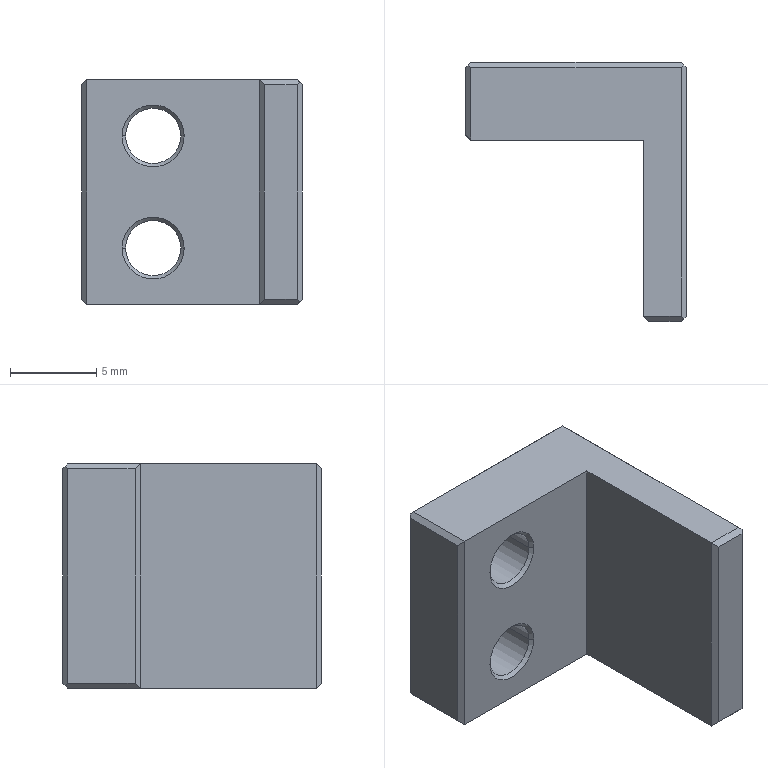Part | NX | 1 solid | 29 faces | box 12.8 x 15 x 13 mm | volume 1011 mm3 | plane 21 | cylinder 4 | cone 4 | commonest cylinder face diameters 3.2 x4
STEP:
#1=CARTESIAN_POINT('',(-175.8,172.2,-82.3));
#2=VERTEX_POINT('',#1);
#3=CARTESIAN_POINT('',(-177.7,172.2,-82.3));
#4=VERTEX_POINT('',#3);
#5=CARTESIAN_POINT('',(-175.,172.2,-82.3));
#6=DIRECTION('',(-1.,0.,0.));
#7=VECTOR('',#6,1000.);
#8=LINE('',#5,#7);
#9=EDGE_CURVE('',#2,#4,#8,.T.);
#10=ORIENTED_EDGE('',*,*,#9,.T.);
#11=CARTESIAN_POINT('',(-177.7,172.2,-94.7));
#12=VERTEX_POINT('',#11);
#13=CARTESIAN_POINT('',(-177.7,172.2,-88.5));
#14=DIRECTION('',(0.,0.,1.));
#15=VECTOR('',#14,1000.);
#16=LINE('',#13,#15);
#17=EDGE_CURVE('',#12,#4,#16,.T.);
#18=ORIENTED_EDGE('',*,*,#17,.F.);
#19=CARTESIAN_POINT('',(-175.8,172.2,-94.7));
#20=VERTEX_POINT('',#19);
#21=CARTESIAN_POINT('',(-175.,172.2,-94.7));
#22=DIRECTION('',(-1.,0.,0.));
#23=VECTOR('',#22,1000.);
#24=LINE('',#21,#23);
#25=EDGE_CURVE('',#20,#12,#24,.T.);
#26=ORIENTED_EDGE('',*,*,#25,.F.);
#27=CARTESIAN_POINT('',(-175.8,172.2,-88.5));
#28=DIRECTION('',(0.,0.,-1.));
#29=VECTOR('',#28,1000.);
#30=LINE('',#27,#29);
#31=EDGE_CURVE('',#2,#20,#30,.T.);
#32=ORIENTED_EDGE('',*,*,#31,.F.);
#33=EDGE_LOOP('',(#10,#18,#26,#32));
#34=FACE_BOUND('',#33,.T.);
#35=CARTESIAN_POINT('',(-175.,172.2,-82.));
#36=DIRECTION('',(0.,-1.,0.));
#37=DIRECTION('',(-1.,0.,0.));
#38=AXIS2_PLACEMENT_3D('',#35,#36,#37);
#39=PLANE('',#38);
#40=ADVANCED_FACE('',(#34),#39,.T.);
#41=CARTESIAN_POINT('',(-175.8,187.2,-94.7));
#42=VERTEX_POINT('',#41);
#43=CARTESIAN_POINT('',(-188.,187.2,-94.7));
#44=VERTEX_POINT('',#43);
#45=CARTESIAN_POINT('',(-175.,187.2,-94.7));
#46=DIRECTION('',(-1.,0.,0.));
#47=VECTOR('',#46,1000.);
#48=LINE('',#45,#47);
#49=EDGE_CURVE('',#42,#44,#48,.T.);
#50=ORIENTED_EDGE('',*,*,#49,.T.);
#51=CARTESIAN_POINT('',(-188.,187.2,-82.3));
#52=VERTEX_POINT('',#51);
#53=CARTESIAN_POINT('',(-188.,187.2,-88.5));
#54=DIRECTION('',(0.,0.,1.));
#55=VECTOR('',#54,1000.);
#56=LINE('',#53,#55);
#57=EDGE_CURVE('',#44,#52,#56,.T.);
#58=ORIENTED_EDGE('',*,*,#57,.T.);
#59=CARTESIAN_POINT('',(-175.8,187.2,-82.3));
#60=VERTEX_POINT('',#59);
#61=CARTESIAN_POINT('',(-175.,187.2,-82.3));
#62=DIRECTION('',(-1.,0.,0.));
#63=VECTOR('',#62,1000.);
#64=LINE('',#61,#63);
#65=EDGE_CURVE('',#60,#52,#64,.T.);
#66=ORIENTED_EDGE('',*,*,#65,.F.);
#67=CARTESIAN_POINT('',(-175.8,187.2,-88.5));
#68=DIRECTION('',(0.,0.,1.));
#69=VECTOR('',#68,1000.);
#70=LINE('',#67,#69);
#71=EDGE_CURVE('',#42,#60,#70,.T.);
#72=ORIENTED_EDGE('',*,*,#71,.F.);
#73=EDGE_LOOP('',(#50,#58,#66,#72));
#74=FACE_BOUND('',#73,.T.);
#75=CARTESIAN_POINT('',(-185.75,187.2,-91.75));
#76=VERTEX_POINT('',#75);
#77=CARTESIAN_POINT('',(-182.55,187.2,-91.75));
#78=VERTEX_POINT('',#77);
#79=CARTESIAN_POINT('',(-184.15,187.2,-91.75));
#80=DIRECTION('',(0.,-1.,0.));
#81=DIRECTION('',(1.,0.,0.));
#82=AXIS2_PLACEMENT_3D('',#79,#80,#81);
#83=CIRCLE('',#82,1.6);
#84=EDGE_CURVE('',#76,#78,#83,.T.);
#85=ORIENTED_EDGE('',*,*,#84,.T.);
#86=CARTESIAN_POINT('',(-184.15,187.2,-91.75));
#87=DIRECTION('',(0.,-1.,0.));
#88=DIRECTION('',(1.,0.,0.));
#89=AXIS2_PLACEMENT_3D('',#86,#87,#88);
#90=CIRCLE('',#89,1.6);
#91=EDGE_CURVE('',#78,#76,#90,.T.);
#92=ORIENTED_EDGE('',*,*,#91,.T.);
#93=EDGE_LOOP('',(#85,#92));
#94=FACE_BOUND('',#93,.T.);
#95=CARTESIAN_POINT('',(-185.75,187.2,-85.25));
#96=VERTEX_POINT('',#95);
#97=CARTESIAN_POINT('',(-182.55,187.2,-85.25));
#98=VERTEX_POINT('',#97);
#99=CARTESIAN_POINT('',(-184.15,187.2,-85.25));
#100=DIRECTION('',(0.,-1.,0.));
#101=DIRECTION('',(1.,0.,0.));
#102=AXIS2_PLACEMENT_3D('',#99,#100,#101);
#103=CIRCLE('',#102,1.6);
#104=EDGE_CURVE('',#96,#98,#103,.T.);
#105=ORIENTED_EDGE('',*,*,#104,.T.);
#106=CARTESIAN_POINT('',(-184.15,187.2,-85.25));
#107=DIRECTION('',(0.,-1.,0.));
#108=DIRECTION('',(1.,0.,0.));
#109=AXIS2_PLACEMENT_3D('',#106,#107,#108);
#110=CIRCLE('',#109,1.6);
#111=EDGE_CURVE('',#98,#96,#110,.T.);
#112=ORIENTED_EDGE('',*,*,#111,.T.);
#113=EDGE_LOOP('',(#105,#112));
#114=FACE_BOUND('',#113,.T.);
#115=CARTESIAN_POINT('',(-190.3,187.2,-95.944));
#116=DIRECTION('',(0.,1.,0.));
#117=DIRECTION('',(0.,0.,-1.));
#118=AXIS2_PLACEMENT_3D('',#115,#116,#117);
#119=PLANE('',#118);
#120=ADVANCED_FACE('',(#74,#94,#114),#119,.T.);
#121=CARTESIAN_POINT('',(-188.3,186.9,-94.7));
#122=VERTEX_POINT('',#121);
#123=CARTESIAN_POINT('',(-188.3,186.9,-82.3));
#124=VERTEX_POINT('',#123);
#125=CARTESIAN_POINT('',(-188.3,186.9,-88.5));
#126=DIRECTION('',(0.,0.,1.));
#127=VECTOR('',#126,1000.);
#128=LINE('',#125,#127);
#129=EDGE_CURVE('',#122,#124,#128,.T.);
#130=ORIENTED_EDGE('',*,*,#129,.F.);
#131=CARTESIAN_POINT('',(-188.3,183.,-94.7));
#132=VERTEX_POINT('',#131);
#133=CARTESIAN_POINT('',(-188.3,184.8,-94.7));
#134=DIRECTION('',(0.,1.,0.));
#135=VECTOR('',#134,1000.);
#136=LINE('',#133,#135);
#137=EDGE_CURVE('',#132,#122,#136,.T.);
#138=ORIENTED_EDGE('',*,*,#137,.F.);
#139=CARTESIAN_POINT('',(-188.3,183.,-82.3));
#140=VERTEX_POINT('',#139);
#141=CARTESIAN_POINT('',(-188.3,183.,-88.5));
#142=DIRECTION('',(0.,0.,-1.));
#143=VECTOR('',#142,1000.);
#144=LINE('',#141,#143);
#145=EDGE_CURVE('',#140,#132,#144,.T.);
#146=ORIENTED_EDGE('',*,*,#145,.F.);
#147=CARTESIAN_POINT('',(-188.3,184.8,-82.3));
#148=DIRECTION('',(0.,1.,0.));
#149=VECTOR('',#148,1000.);
#150=LINE('',#147,#149);
#151=EDGE_CURVE('',#140,#124,#150,.T.);
#152=ORIENTED_EDGE('',*,*,#151,.T.);
#153=EDGE_LOOP('',(#130,#138,#146,#152));
#154=FACE_BOUND('',#153,.T.);
#155=CARTESIAN_POINT('',(-188.3,182.7,-95.944));
#156=DIRECTION('',(-1.,0.,0.));
#157=DIRECTION('',(0.,1.,0.));
#158=AXIS2_PLACEMENT_3D('',#155,#156,#157);
#159=PLANE('',#158);
#160=ADVANCED_FACE('',(#154),#159,.T.);
#161=CARTESIAN_POINT('',(-175.8,172.5,-95.));
#162=VERTEX_POINT('',#161);
#163=CARTESIAN_POINT('',(-178.,172.5,-95.));
#164=VERTEX_POINT('',#163);
#165=CARTESIAN_POINT('',(-175.,172.5,-95.));
#166=DIRECTION('',(-1.,0.,0.));
#167=VECTOR('',#166,1000.);
#168=LINE('',#165,#167);
#169=EDGE_CURVE('',#162,#164,#168,.T.);
#170=ORIENTED_EDGE('',*,*,#169,.T.);
#171=CARTESIAN_POINT('',(-178.,182.7,-95.));
#172=VERTEX_POINT('',#171);
#173=CARTESIAN_POINT('',(-178.,180.866,-95.));
#174=DIRECTION('',(0.,-1.,0.));
#175=VECTOR('',#174,1000.);
#176=LINE('',#173,#175);
#177=EDGE_CURVE('',#172,#164,#176,.T.);
#178=ORIENTED_EDGE('',*,*,#177,.F.);
#179=CARTESIAN_POINT('',(-188.,182.7,-95.));
#180=VERTEX_POINT('',#179);
#181=CARTESIAN_POINT('',(-175.,182.7,-95.));
#182=DIRECTION('',(1.,0.,0.));
#183=VECTOR('',#182,1000.);
#184=LINE('',#181,#183);
#185=EDGE_CURVE('',#180,#172,#184,.T.);
#186=ORIENTED_EDGE('',*,*,#185,.F.);
#187=CARTESIAN_POINT('',(-188.,186.9,-95.));
#188=VERTEX_POINT('',#187);
#189=CARTESIAN_POINT('',(-188.,184.8,-95.));
#190=DIRECTION('',(0.,1.,0.));
#191=VECTOR('',#190,1000.);
#192=LINE('',#189,#191);
#193=EDGE_CURVE('',#180,#188,#192,.T.);
#194=ORIENTED_EDGE('',*,*,#193,.T.);
#195=CARTESIAN_POINT('',(-175.8,186.9,-95.));
#196=VERTEX_POINT('',#195);
#197=CARTESIAN_POINT('',(-175.,186.9,-95.));
#198=DIRECTION('',(-1.,0.,0.));
#199=VECTOR('',#198,1000.);
#200=LINE('',#197,#199);
#201=EDGE_CURVE('',#196,#188,#200,.T.);
#202=ORIENTED_EDGE('',*,*,#201,.F.);
#203=CARTESIAN_POINT('',(-175.8,179.7,-95.));
#204=DIRECTION('',(0.,1.,0.));
#205=VECTOR('',#204,1000.);
#206=LINE('',#203,#205);
#207=EDGE_CURVE('',#162,#196,#206,.T.);
#208=ORIENTED_EDGE('',*,*,#207,.F.);
#209=EDGE_LOOP('',(#170,#178,#186,#194,#202,#208));
#210=FACE_BOUND('',#209,.T.);
#211=CARTESIAN_POINT('',(-176.432,184.505,-95.));
#212=DIRECTION('',(0.,0.,-1.));
#213=DIRECTION('',(-1.,0.,0.));
#214=AXIS2_PLACEMENT_3D('',#211,#212,#213);
#215=PLANE('',#214);
#216=ADVANCED_FACE('',(#210),#215,.T.);
#217=ORIENTED_EDGE('',*,*,#185,.T.);
#218=CARTESIAN_POINT('',(-178.,182.7,-82.));
#219=VERTEX_POINT('',#218);
#220=CARTESIAN_POINT('',(-178.,182.7,-87.033));
#221=DIRECTION('',(0.,0.,1.));
#222=VECTOR('',#221,1000.);
#223=LINE('',#220,#222);
#224=EDGE_CURVE('',#172,#219,#223,.T.);
#225=ORIENTED_EDGE('',*,*,#224,.T.);
#226=CARTESIAN_POINT('',(-188.,182.7,-82.));
#227=VERTEX_POINT('',#226);
#228=CARTESIAN_POINT('',(-175.,182.7,-82.));
#229=DIRECTION('',(1.,0.,0.));
#230=VECTOR('',#229,1000.);
#231=LINE('',#228,#230);
#232=EDGE_CURVE('',#227,#219,#231,.T.);
#233=ORIENTED_EDGE('',*,*,#232,.F.);
#234=CARTESIAN_POINT('',(-188.,182.7,-88.5));
#235=DIRECTION('',(0.,0.,-1.));
#236=VECTOR('',#235,1000.);
#237=LINE('',#234,#236);
#238=EDGE_CURVE('',#227,#180,#237,.T.);
#239=ORIENTED_EDGE('',*,*,#238,.T.);
#240=EDGE_LOOP('',(#217,#225,#233,#239));
#241=FACE_BOUND('',#240,.T.);
#242=CARTESIAN_POINT('',(-185.95,182.7,-85.25));
#243=VERTEX_POINT('',#242);
#244=CARTESIAN_POINT('',(-182.35,182.7,-85.25));
#245=VERTEX_POINT('',#244);
#246=CARTESIAN_POINT('',(-184.15,182.7,-85.25));
#247=DIRECTION('',(0.,-1.,0.));
#248=DIRECTION('',(1.,0.,0.));
#249=AXIS2_PLACEMENT_3D('',#246,#247,#248);
#250=CIRCLE('',#249,1.8);
#251=EDGE_CURVE('',#243,#245,#250,.T.);
#252=ORIENTED_EDGE('',*,*,#251,.F.);
#253=CARTESIAN_POINT('',(-184.15,182.7,-85.25));
#254=DIRECTION('',(0.,-1.,0.));
#255=DIRECTION('',(1.,0.,0.));
#256=AXIS2_PLACEMENT_3D('',#253,#254,#255);
#257=CIRCLE('',#256,1.8);
#258=EDGE_CURVE('',#245,#243,#257,.T.);
#259=ORIENTED_EDGE('',*,*,#258,.F.);
#260=EDGE_LOOP('',(#252,#259));
#261=FACE_BOUND('',#260,.T.);
#262=CARTESIAN_POINT('',(-185.95,182.7,-91.75));
#263=VERTEX_POINT('',#262);
#264=CARTESIAN_POINT('',(-182.35,182.7,-91.75));
#265=VERTEX_POINT('',#264);
#266=CARTESIAN_POINT('',(-184.15,182.7,-91.75));
#267=DIRECTION('',(0.,-1.,0.));
#268=DIRECTION('',(1.,0.,0.));
#269=AXIS2_PLACEMENT_3D('',#266,#267,#268);
#270=CIRCLE('',#269,1.8);
#271=EDGE_CURVE('',#263,#265,#270,.T.);
#272=ORIENTED_EDGE('',*,*,#271,.F.);
#273=CARTESIAN_POINT('',(-184.15,182.7,-91.75));
#274=DIRECTION('',(0.,-1.,0.));
#275=DIRECTION('',(1.,0.,0.));
#276=AXIS2_PLACEMENT_3D('',#273,#274,#275);
#277=CIRCLE('',#276,1.8);
#278=EDGE_CURVE('',#265,#263,#277,.T.);
#279=ORIENTED_EDGE('',*,*,#278,.F.);
#280=EDGE_LOOP('',(#272,#279));
#281=FACE_BOUND('',#280,.T.);
#282=CARTESIAN_POINT('',(-178.,182.7,-95.944));
#283=DIRECTION('',(0.,-1.,0.));
#284=DIRECTION('',(0.,0.,-1.));
#285=AXIS2_PLACEMENT_3D('',#282,#283,#284);
#286=PLANE('',#285);
#287=ADVANCED_FACE('',(#241,#261,#281),#286,.T.);
#288=CARTESIAN_POINT('',(-175.8,172.5,-82.));
#289=VERTEX_POINT('',#288);
#290=CARTESIAN_POINT('',(-175.8,186.9,-82.));
#291=VERTEX_POINT('',#290);
#292=CARTESIAN_POINT('',(-175.8,179.7,-82.));
#293=DIRECTION('',(0.,1.,0.));
#294=VECTOR('',#293,1000.);
#295=LINE('',#292,#294);
#296=EDGE_CURVE('',#289,#291,#295,.T.);
#297=ORIENTED_EDGE('',*,*,#296,.T.);
#298=CARTESIAN_POINT('',(-188.,186.9,-82.));
#299=VERTEX_POINT('',#298);
#300=CARTESIAN_POINT('',(-175.,186.9,-82.));
#301=DIRECTION('',(-1.,0.,0.));
#302=VECTOR('',#301,1000.);
#303=LINE('',#300,#302);
#304=EDGE_CURVE('',#291,#299,#303,.T.);
#305=ORIENTED_EDGE('',*,*,#304,.T.);
#306=CARTESIAN_POINT('',(-188.,184.8,-82.));
#307=DIRECTION('',(0.,1.,0.));
#308=VECTOR('',#307,1000.);
#309=LINE('',#306,#308);
#310=EDGE_CURVE('',#227,#299,#309,.T.);
#311=ORIENTED_EDGE('',*,*,#310,.F.);
#312=ORIENTED_EDGE('',*,*,#232,.T.);
#313=CARTESIAN_POINT('',(-178.,172.5,-82.));
#314=VERTEX_POINT('',#313);
#315=CARTESIAN_POINT('',(-178.,180.866,-82.));
#316=DIRECTION('',(0.,-1.,0.));
#317=VECTOR('',#316,1000.);
#318=LINE('',#315,#317);
#319=EDGE_CURVE('',#219,#314,#318,.T.);
#320=ORIENTED_EDGE('',*,*,#319,.T.);
#321=CARTESIAN_POINT('',(-175.,172.5,-82.));
#322=DIRECTION('',(-1.,0.,0.));
#323=VECTOR('',#322,1000.);
#324=LINE('',#321,#323);
#325=EDGE_CURVE('',#289,#314,#324,.T.);
#326=ORIENTED_EDGE('',*,*,#325,.F.);
#327=EDGE_LOOP('',(#297,#305,#311,#312,#320,#326));
#328=FACE_BOUND('',#327,.T.);
#329=CARTESIAN_POINT('',(-176.432,184.505,-82.));
#330=DIRECTION('',(0.,0.,-1.));
#331=DIRECTION('',(-1.,0.,0.));
#332=AXIS2_PLACEMENT_3D('',#329,#330,#331);
#333=PLANE('',#332);
#334=ADVANCED_FACE('',(#328),#333,.F.);
#335=CARTESIAN_POINT('',(-185.75,182.9,-85.25));
#336=VERTEX_POINT('',#335);
#337=CARTESIAN_POINT('',(-182.55,182.9,-85.25));
#338=VERTEX_POINT('',#337);
#339=CARTESIAN_POINT('',(-184.15,182.9,-85.25));
#340=DIRECTION('',(0.,-1.,0.));
#341=DIRECTION('',(1.,0.,0.));
#342=AXIS2_PLACEMENT_3D('',#339,#340,#341);
#343=CIRCLE('',#342,1.6);
#344=EDGE_CURVE('',#336,#338,#343,.T.);
#345=ORIENTED_EDGE('',*,*,#344,.T.);
#346=CARTESIAN_POINT('',(-182.55,182.7,-85.25));
#347=DIRECTION('',(0.,-1.,0.));
#348=VECTOR('',#347,1000.);
#349=LINE('',#346,#348);
#350=EDGE_CURVE('',#98,#338,#349,.T.);
#351=ORIENTED_EDGE('',*,*,#350,.F.);
#352=ORIENTED_EDGE('',*,*,#104,.F.);
#353=CARTESIAN_POINT('',(-185.75,182.7,-85.25));
#354=DIRECTION('',(0.,-1.,0.));
#355=VECTOR('',#354,1000.);
#356=LINE('',#353,#355);
#357=EDGE_CURVE('',#96,#336,#356,.T.);
#358=ORIENTED_EDGE('',*,*,#357,.T.);
#359=EDGE_LOOP('',(#345,#351,#352,#358));
#360=FACE_BOUND('',#359,.T.);
#361=CARTESIAN_POINT('',(-184.15,182.7,-85.25));
#362=DIRECTION('',(0.,-1.,0.));
#363=DIRECTION('',(1.,0.,0.));
#364=AXIS2_PLACEMENT_3D('',#361,#362,#363);
#365=CYLINDRICAL_SURFACE('',#364,1.6);
#366=ADVANCED_FACE('',(#360),#365,.F.);
#367=ORIENTED_EDGE('',*,*,#344,.F.);
#368=CARTESIAN_POINT('',(-185.75,182.9,-85.25));
#369=DIRECTION('',(-0.7071,-0.7071,0.));
#370=VECTOR('',#369,1000.);
#371=LINE('',#368,#370);
#372=EDGE_CURVE('',#336,#243,#371,.T.);
#373=ORIENTED_EDGE('',*,*,#372,.T.);
#374=ORIENTED_EDGE('',*,*,#251,.T.);
#375=CARTESIAN_POINT('',(-182.55,182.9,-85.25));
#376=DIRECTION('',(0.7071,-0.7071,0.));
#377=VECTOR('',#376,1000.);
#378=LINE('',#375,#377);
#379=EDGE_CURVE('',#338,#245,#378,.T.);
#380=ORIENTED_EDGE('',*,*,#379,.F.);
#381=EDGE_LOOP('',(#367,#373,#374,#380));
#382=FACE_BOUND('',#381,.T.);
#383=CARTESIAN_POINT('',(-184.15,182.9,-85.25));
#384=DIRECTION('',(0.,-1.,0.));
#385=DIRECTION('',(1.,0.,0.));
#386=AXIS2_PLACEMENT_3D('',#383,#384,#385);
#387=CONICAL_SURFACE('',#386,1.6,0.7854);
#388=ADVANCED_FACE('',(#382),#387,.F.);
#389=CARTESIAN_POINT('',(-185.75,182.9,-91.75));
#390=VERTEX_POINT('',#389);
#391=CARTESIAN_POINT('',(-182.55,182.9,-91.75));
#392=VERTEX_POINT('',#391);
#393=CARTESIAN_POINT('',(-184.15,182.9,-91.75));
#394=DIRECTION('',(0.,-1.,0.));
#395=DIRECTION('',(1.,0.,0.));
#396=AXIS2_PLACEMENT_3D('',#393,#394,#395);
#397=CIRCLE('',#396,1.6);
#398=EDGE_CURVE('',#390,#392,#397,.T.);
#399=ORIENTED_EDGE('',*,*,#398,.T.);
#400=CARTESIAN_POINT('',(-182.55,182.7,-91.75));
#401=DIRECTION('',(0.,-1.,0.));
#402=VECTOR('',#401,1000.);
#403=LINE('',#400,#402);
#404=EDGE_CURVE('',#78,#392,#403,.T.);
#405=ORIENTED_EDGE('',*,*,#404,.F.);
#406=ORIENTED_EDGE('',*,*,#84,.F.);
#407=CARTESIAN_POINT('',(-185.75,182.7,-91.75));
#408=DIRECTION('',(0.,-1.,0.));
#409=VECTOR('',#408,1000.);
#410=LINE('',#407,#409);
#411=EDGE_CURVE('',#76,#390,#410,.T.);
#412=ORIENTED_EDGE('',*,*,#411,.T.);
#413=EDGE_LOOP('',(#399,#405,#406,#412));
#414=FACE_BOUND('',#413,.T.);
#415=CARTESIAN_POINT('',(-184.15,182.7,-91.75));
#416=DIRECTION('',(0.,-1.,0.));
#417=DIRECTION('',(1.,0.,0.));
#418=AXIS2_PLACEMENT_3D('',#415,#416,#417);
#419=CYLINDRICAL_SURFACE('',#418,1.6);
#420=ADVANCED_FACE('',(#414),#419,.F.);
#421=ORIENTED_EDGE('',*,*,#398,.F.);
#422=CARTESIAN_POINT('',(-185.75,182.9,-91.75));
#423=DIRECTION('',(-0.7071,-0.7071,0.));
#424=VECTOR('',#423,1000.);
#425=LINE('',#422,#424);
#426=EDGE_CURVE('',#390,#263,#425,.T.);
#427=ORIENTED_EDGE('',*,*,#426,.T.);
#428=ORIENTED_EDGE('',*,*,#271,.T.);
#429=CARTESIAN_POINT('',(-182.55,182.9,-91.75));
#430=DIRECTION('',(0.7071,-0.7071,0.));
#431=VECTOR('',#430,1000.);
#432=LINE('',#429,#431);
#433=EDGE_CURVE('',#392,#265,#432,.T.);
#434=ORIENTED_EDGE('',*,*,#433,.F.);
#435=EDGE_LOOP('',(#421,#427,#428,#434));
#436=FACE_BOUND('',#435,.T.);
#437=CARTESIAN_POINT('',(-184.15,182.9,-91.75));
#438=DIRECTION('',(0.,-1.,0.));
#439=DIRECTION('',(1.,0.,0.));
#440=AXIS2_PLACEMENT_3D('',#437,#438,#439);
#441=CONICAL_SURFACE('',#440,1.6,0.7854);
#442=ADVANCED_FACE('',(#436),#441,.F.);
#443=ORIENTED_EDGE('',*,*,#169,.F.);
#444=CARTESIAN_POINT('',(-175.65,172.35,-94.85));
#445=VERTEX_POINT('',#444);
#446=CARTESIAN_POINT('',(-184.166,180.866,-103.366));
#447=DIRECTION('',(0.5774,-0.5774,0.5774));
#448=VECTOR('',#447,1000.);
#449=LINE('',#446,#448);
#450=EDGE_CURVE('',#162,#445,#449,.T.);
#451=ORIENTED_EDGE('',*,*,#450,.T.);
#452=CARTESIAN_POINT('',(-167.134,180.866,-103.366));
#453=DIRECTION('',(-0.5774,-0.5774,0.5774));
#454=VECTOR('',#453,1000.);
#455=LINE('',#452,#454);
#456=EDGE_CURVE('',#445,#20,#455,.T.);
#457=ORIENTED_EDGE('',*,*,#456,.T.);
#458=ORIENTED_EDGE('',*,*,#25,.T.);
#459=CARTESIAN_POINT('',(-186.366,180.866,-103.366));
#460=DIRECTION('',(-0.5774,0.5774,-0.5774));
#461=VECTOR('',#460,1000.);
#462=LINE('',#459,#461);
#463=EDGE_CURVE('',#12,#164,#462,.T.);
#464=ORIENTED_EDGE('',*,*,#463,.T.);
#465=EDGE_LOOP('',(#443,#451,#457,#458,#464));
#466=FACE_BOUND('',#465,.T.);
#467=CARTESIAN_POINT('',(-176.5,172.35,-94.85));
#468=DIRECTION('',(0.,0.7071,0.7071));
#469=DIRECTION('',(1.,0.,0.));
#470=AXIS2_PLACEMENT_3D('',#467,#468,#469);
#471=PLANE('',#470);
#472=ADVANCED_FACE('',(#466),#471,.F.);
#473=ORIENTED_EDGE('',*,*,#49,.F.);
#474=CARTESIAN_POINT('',(-175.65,187.05,-94.85));
#475=VERTEX_POINT('',#474);
#476=CARTESIAN_POINT('',(-175.,186.4,-95.5));
#477=DIRECTION('',(0.5774,-0.5774,-0.5774));
#478=VECTOR('',#477,1000.);
#479=LINE('',#476,#478);
#480=EDGE_CURVE('',#42,#475,#479,.T.);
#481=ORIENTED_EDGE('',*,*,#480,.T.);
#482=CARTESIAN_POINT('',(-181.834,180.866,-101.034));
#483=DIRECTION('',(-0.5774,-0.5774,-0.5774));
#484=VECTOR('',#483,1000.);
#485=LINE('',#482,#484);
#486=EDGE_CURVE('',#475,#196,#485,.T.);
#487=ORIENTED_EDGE('',*,*,#486,.T.);
#488=ORIENTED_EDGE('',*,*,#201,.T.);
#489=CARTESIAN_POINT('',(-188.15,187.05,-94.85));
#490=VERTEX_POINT('',#489);
#491=CARTESIAN_POINT('',(-175.,173.9,-108.));
#492=DIRECTION('',(-0.5774,0.5774,0.5774));
#493=VECTOR('',#492,1000.);
#494=LINE('',#491,#493);
#495=EDGE_CURVE('',#188,#490,#494,.T.);
#496=ORIENTED_EDGE('',*,*,#495,.T.);
#497=CARTESIAN_POINT('',(-194.334,180.866,-101.034));
#498=DIRECTION('',(-0.5774,-0.5774,-0.5774));
#499=VECTOR('',#498,1000.);
#500=LINE('',#497,#499);
#501=EDGE_CURVE('',#44,#490,#500,.T.);
#502=ORIENTED_EDGE('',*,*,#501,.F.);
#503=EDGE_LOOP('',(#473,#481,#487,#488,#496,#502));
#504=FACE_BOUND('',#503,.T.);
#505=CARTESIAN_POINT('',(-182.65,187.05,-94.85));
#506=DIRECTION('',(0.,-0.7071,0.7071));
#507=DIRECTION('',(-1.,0.,0.));
#508=AXIS2_PLACEMENT_3D('',#505,#506,#507);
#509=PLANE('',#508);
#510=ADVANCED_FACE('',(#504),#509,.F.);
#511=ORIENTED_EDGE('',*,*,#304,.F.);
#512=CARTESIAN_POINT('',(-175.65,187.05,-82.15));
#513=VERTEX_POINT('',#512);
#514=CARTESIAN_POINT('',(-175.,187.7,-82.8));
#515=DIRECTION('',(0.5774,0.5773,-0.5774));
#516=VECTOR('',#515,1000.);
#517=LINE('',#514,#516);
#518=EDGE_CURVE('',#291,#513,#517,.T.);
#519=ORIENTED_EDGE('',*,*,#518,.T.);
#520=CARTESIAN_POINT('',(-180.533,191.933,-87.033));
#521=DIRECTION('',(0.5773,-0.5773,0.5774));
#522=VECTOR('',#521,1000.);
#523=LINE('',#520,#522);
#524=EDGE_CURVE('',#60,#513,#523,.T.);
#525=ORIENTED_EDGE('',*,*,#524,.F.);
#526=ORIENTED_EDGE('',*,*,#65,.T.);
#527=CARTESIAN_POINT('',(-188.15,187.05,-82.15));
#528=VERTEX_POINT('',#527);
#529=CARTESIAN_POINT('',(-183.267,191.933,-87.033));
#530=DIRECTION('',(-0.5773,-0.5773,0.5774));
#531=VECTOR('',#530,1000.);
#532=LINE('',#529,#531);
#533=EDGE_CURVE('',#52,#528,#532,.T.);
#534=ORIENTED_EDGE('',*,*,#533,.T.);
#535=CARTESIAN_POINT('',(-175.,173.9,-69.));
#536=DIRECTION('',(0.5774,-0.5773,0.5774));
#537=VECTOR('',#536,1000.);
#538=LINE('',#535,#537);
#539=EDGE_CURVE('',#528,#299,#538,.T.);
#540=ORIENTED_EDGE('',*,*,#539,.T.);
#541=EDGE_LOOP('',(#511,#519,#525,#526,#534,#540));
#542=FACE_BOUND('',#541,.T.);
#543=CARTESIAN_POINT('',(-182.65,187.05,-82.15));
#544=DIRECTION('',(0.,0.7071,0.7071));
#545=DIRECTION('',(1.,0.,0.));
#546=AXIS2_PLACEMENT_3D('',#543,#544,#545);
#547=PLANE('',#546);
#548=ADVANCED_FACE('',(#542),#547,.T.);
#549=ORIENTED_EDGE('',*,*,#9,.F.);
#550=CARTESIAN_POINT('',(-175.65,172.35,-82.15));
#551=VERTEX_POINT('',#550);
#552=CARTESIAN_POINT('',(-167.134,180.866,-73.634));
#553=DIRECTION('',(-0.5774,-0.5774,-0.5774));
#554=VECTOR('',#553,1000.);
#555=LINE('',#552,#554);
#556=EDGE_CURVE('',#551,#2,#555,.T.);
#557=ORIENTED_EDGE('',*,*,#556,.F.);
#558=CARTESIAN_POINT('',(-184.166,180.866,-73.634));
#559=DIRECTION('',(-0.5774,0.5774,0.5774));
#560=VECTOR('',#559,1000.);
#561=LINE('',#558,#560);
#562=EDGE_CURVE('',#551,#289,#561,.T.);
#563=ORIENTED_EDGE('',*,*,#562,.T.);
#564=ORIENTED_EDGE('',*,*,#325,.T.);
#565=CARTESIAN_POINT('',(-186.366,180.866,-73.634));
#566=DIRECTION('',(-0.5774,0.5774,0.5774));
#567=VECTOR('',#566,1000.);
#568=LINE('',#565,#567);
#569=EDGE_CURVE('',#4,#314,#568,.T.);
#570=ORIENTED_EDGE('',*,*,#569,.F.);
#571=EDGE_LOOP('',(#549,#557,#563,#564,#570));
#572=FACE_BOUND('',#571,.T.);
#573=CARTESIAN_POINT('',(-176.5,172.35,-82.15));
#574=DIRECTION('',(0.,-0.7071,0.7071));
#575=DIRECTION('',(-1.,0.,0.));
#576=AXIS2_PLACEMENT_3D('',#573,#574,#575);
#577=PLANE('',#576);
#578=ADVANCED_FACE('',(#572),#577,.T.);
#579=ORIENTED_EDGE('',*,*,#145,.T.);
#580=CARTESIAN_POINT('',(-175.,169.7,-108.));
#581=DIRECTION('',(-0.5774,0.5774,0.5774));
#582=VECTOR('',#581,1000.);
#583=LINE('',#580,#582);
#584=EDGE_CURVE('',#180,#132,#583,.T.);
#585=ORIENTED_EDGE('',*,*,#584,.F.);
#586=ORIENTED_EDGE('',*,*,#238,.F.);
#587=CARTESIAN_POINT('',(-175.,169.7,-69.));
#588=DIRECTION('',(-0.5774,0.5774,-0.5774));
#589=VECTOR('',#588,1000.);
#590=LINE('',#587,#589);
#591=EDGE_CURVE('',#227,#140,#590,.T.);
#592=ORIENTED_EDGE('',*,*,#591,.T.);
#593=EDGE_LOOP('',(#579,#585,#586,#592));
#594=FACE_BOUND('',#593,.T.);
#595=CARTESIAN_POINT('',(-188.15,182.85,-88.5));
#596=DIRECTION('',(0.7071,0.7071,0.));
#597=DIRECTION('',(0.,0.,-1.));
#598=AXIS2_PLACEMENT_3D('',#595,#596,#597);
#599=PLANE('',#598);
#600=ADVANCED_FACE('',(#594),#599,.F.);
#601=ORIENTED_EDGE('',*,*,#193,.F.);
#602=ORIENTED_EDGE('',*,*,#584,.T.);
#603=ORIENTED_EDGE('',*,*,#137,.T.);
#604=CARTESIAN_POINT('',(-194.334,180.866,-88.666));
#605=DIRECTION('',(0.5774,0.5774,-0.5774));
#606=VECTOR('',#605,1000.);
#607=LINE('',#604,#606);
#608=EDGE_CURVE('',#122,#490,#607,.T.);
#609=ORIENTED_EDGE('',*,*,#608,.T.);
#610=ORIENTED_EDGE('',*,*,#495,.F.);
#611=EDGE_LOOP('',(#601,#602,#603,#609,#610));
#612=FACE_BOUND('',#611,.T.);
#613=CARTESIAN_POINT('',(-188.15,184.8,-94.85));
#614=DIRECTION('',(-0.7071,0.,-0.7071));
#615=DIRECTION('',(-0.7071,0.,0.7071));
#616=AXIS2_PLACEMENT_3D('',#613,#614,#615);
#617=PLANE('',#616);
#618=ADVANCED_FACE('',(#612),#617,.T.);
#619=ORIENTED_EDGE('',*,*,#129,.T.);
#620=CARTESIAN_POINT('',(-194.334,180.866,-88.334));
#621=DIRECTION('',(-0.5774,-0.5774,-0.5774));
#622=VECTOR('',#621,1000.);
#623=LINE('',#620,#622);
#624=EDGE_CURVE('',#528,#124,#623,.T.);
#625=ORIENTED_EDGE('',*,*,#624,.F.);
#626=ORIENTED_EDGE('',*,*,#533,.F.);
#627=ORIENTED_EDGE('',*,*,#57,.F.);
#628=ORIENTED_EDGE('',*,*,#501,.T.);
#629=ORIENTED_EDGE('',*,*,#608,.F.);
#630=EDGE_LOOP('',(#619,#625,#626,#627,#628,#629));
#631=FACE_BOUND('',#630,.T.);
#632=CARTESIAN_POINT('',(-188.15,187.05,-88.5));
#633=DIRECTION('',(0.7071,-0.7071,0.));
#634=DIRECTION('',(0.,0.,-1.));
#635=AXIS2_PLACEMENT_3D('',#632,#633,#634);
#636=PLANE('',#635);
#637=ADVANCED_FACE('',(#631),#636,.F.);
#638=ORIENTED_EDGE('',*,*,#310,.T.);
#639=ORIENTED_EDGE('',*,*,#539,.F.);
#640=ORIENTED_EDGE('',*,*,#624,.T.);
#641=ORIENTED_EDGE('',*,*,#151,.F.);
#642=ORIENTED_EDGE('',*,*,#591,.F.);
#643=EDGE_LOOP('',(#638,#639,#640,#641,#642));
#644=FACE_BOUND('',#643,.T.);
#645=CARTESIAN_POINT('',(-188.15,184.8,-82.15));
#646=DIRECTION('',(0.7071,0.,-0.7071));
#647=DIRECTION('',(0.,-1.,0.));
#648=AXIS2_PLACEMENT_3D('',#645,#646,#647);
#649=PLANE('',#648);
#650=ADVANCED_FACE('',(#644),#649,.F.);
#651=ORIENTED_EDGE('',*,*,#404,.T.);
#652=CARTESIAN_POINT('',(-184.15,182.9,-91.75));
#653=DIRECTION('',(0.,-1.,0.));
#654=DIRECTION('',(1.,0.,0.));
#655=AXIS2_PLACEMENT_3D('',#652,#653,#654);
#656=CIRCLE('',#655,1.6);
#657=EDGE_CURVE('',#392,#390,#656,.T.);
#658=ORIENTED_EDGE('',*,*,#657,.T.);
#659=ORIENTED_EDGE('',*,*,#411,.F.);
#660=ORIENTED_EDGE('',*,*,#91,.F.);
#661=EDGE_LOOP('',(#651,#658,#659,#660));
#662=FACE_BOUND('',#661,.T.);
#663=CARTESIAN_POINT('',(-184.15,182.7,-91.75));
#664=DIRECTION('',(0.,-1.,0.));
#665=DIRECTION('',(1.,0.,0.));
#666=AXIS2_PLACEMENT_3D('',#663,#664,#665);
#667=CYLINDRICAL_SURFACE('',#666,1.6);
#668=ADVANCED_FACE('',(#662),#667,.F.);
#669=ORIENTED_EDGE('',*,*,#433,.T.);
#670=ORIENTED_EDGE('',*,*,#278,.T.);
#671=ORIENTED_EDGE('',*,*,#426,.F.);
#672=ORIENTED_EDGE('',*,*,#657,.F.);
#673=EDGE_LOOP('',(#669,#670,#671,#672));
#674=FACE_BOUND('',#673,.T.);
#675=CARTESIAN_POINT('',(-184.15,182.9,-91.75));
#676=DIRECTION('',(0.,-1.,0.));
#677=DIRECTION('',(1.,0.,0.));
#678=AXIS2_PLACEMENT_3D('',#675,#676,#677);
#679=CONICAL_SURFACE('',#678,1.6,0.7854);
#680=ADVANCED_FACE('',(#674),#679,.F.);
#681=ORIENTED_EDGE('',*,*,#350,.T.);
#682=CARTESIAN_POINT('',(-184.15,182.9,-85.25));
#683=DIRECTION('',(0.,-1.,0.));
#684=DIRECTION('',(1.,0.,0.));
#685=AXIS2_PLACEMENT_3D('',#682,#683,#684);
#686=CIRCLE('',#685,1.6);
#687=EDGE_CURVE('',#338,#336,#686,.T.);
#688=ORIENTED_EDGE('',*,*,#687,.T.);
#689=ORIENTED_EDGE('',*,*,#357,.F.);
#690=ORIENTED_EDGE('',*,*,#111,.F.);
#691=EDGE_LOOP('',(#681,#688,#689,#690));
#692=FACE_BOUND('',#691,.T.);
#693=CARTESIAN_POINT('',(-184.15,182.7,-85.25));
#694=DIRECTION('',(0.,-1.,0.));
#695=DIRECTION('',(1.,0.,0.));
#696=AXIS2_PLACEMENT_3D('',#693,#694,#695);
#697=CYLINDRICAL_SURFACE('',#696,1.6);
#698=ADVANCED_FACE('',(#692),#697,.F.);
#699=ORIENTED_EDGE('',*,*,#379,.T.);
#700=ORIENTED_EDGE('',*,*,#258,.T.);
#701=ORIENTED_EDGE('',*,*,#372,.F.);
#702=ORIENTED_EDGE('',*,*,#687,.F.);
#703=EDGE_LOOP('',(#699,#700,#701,#702));
#704=FACE_BOUND('',#703,.T.);
#705=CARTESIAN_POINT('',(-184.15,182.9,-85.25));
#706=DIRECTION('',(0.,-1.,0.));
#707=DIRECTION('',(1.,0.,0.));
#708=AXIS2_PLACEMENT_3D('',#705,#706,#707);
#709=CONICAL_SURFACE('',#708,1.6,0.7854);
#710=ADVANCED_FACE('',(#704),#709,.F.);
#711=CARTESIAN_POINT('',(-178.,172.5,-88.5));
#712=DIRECTION('',(0.,0.,1.));
#713=VECTOR('',#712,1000.);
#714=LINE('',#711,#713);
#715=EDGE_CURVE('',#164,#314,#714,.T.);
#716=ORIENTED_EDGE('',*,*,#715,.T.);
#717=ORIENTED_EDGE('',*,*,#319,.F.);
#718=ORIENTED_EDGE('',*,*,#224,.F.);
#719=ORIENTED_EDGE('',*,*,#177,.T.);
#720=EDGE_LOOP('',(#716,#717,#718,#719));
#721=FACE_BOUND('',#720,.T.);
#722=CARTESIAN_POINT('',(-178.,180.866,-87.033));
#723=DIRECTION('',(-1.,0.,0.));
#724=DIRECTION('',(0.,0.,1.));
#725=AXIS2_PLACEMENT_3D('',#722,#723,#724);
#726=PLANE('',#725);
#727=ADVANCED_FACE('',(#721),#726,.T.);
#728=ORIENTED_EDGE('',*,*,#715,.F.);
#729=ORIENTED_EDGE('',*,*,#463,.F.);
#730=ORIENTED_EDGE('',*,*,#17,.T.);
#731=ORIENTED_EDGE('',*,*,#569,.T.);
#732=EDGE_LOOP('',(#728,#729,#730,#731));
#733=FACE_BOUND('',#732,.T.);
#734=CARTESIAN_POINT('',(-177.85,172.35,-88.5));
#735=DIRECTION('',(-0.7071,-0.7071,0.));
#736=DIRECTION('',(-0.7071,0.7071,0.));
#737=AXIS2_PLACEMENT_3D('',#734,#735,#736);
#738=PLANE('',#737);
#739=ADVANCED_FACE('',(#733),#738,.T.);
#740=CARTESIAN_POINT('',(-175.5,172.5,-82.3));
#741=VERTEX_POINT('',#740);
#742=CARTESIAN_POINT('',(-175.5,172.5,-94.7));
#743=VERTEX_POINT('',#742);
#744=CARTESIAN_POINT('',(-175.5,172.5,-88.5));
#745=DIRECTION('',(0.,0.,-1.));
#746=VECTOR('',#745,1000.);
#747=LINE('',#744,#746);
#748=EDGE_CURVE('',#741,#743,#747,.T.);
#749=ORIENTED_EDGE('',*,*,#748,.T.);
#750=CARTESIAN_POINT('',(-175.5,186.9,-94.7));
#751=VERTEX_POINT('',#750);
#752=CARTESIAN_POINT('',(-175.5,179.7,-94.7));
#753=DIRECTION('',(0.,1.,0.));
#754=VECTOR('',#753,1000.);
#755=LINE('',#752,#754);
#756=EDGE_CURVE('',#743,#751,#755,.T.);
#757=ORIENTED_EDGE('',*,*,#756,.T.);
#758=CARTESIAN_POINT('',(-175.5,186.9,-82.3));
#759=VERTEX_POINT('',#758);
#760=CARTESIAN_POINT('',(-175.5,186.9,-88.5));
#761=DIRECTION('',(0.,0.,1.));
#762=VECTOR('',#761,1000.);
#763=LINE('',#760,#762);
#764=EDGE_CURVE('',#751,#759,#763,.T.);
#765=ORIENTED_EDGE('',*,*,#764,.T.);
#766=CARTESIAN_POINT('',(-175.5,179.7,-82.3));
#767=DIRECTION('',(0.,1.,0.));
#768=VECTOR('',#767,1000.);
#769=LINE('',#766,#768);
#770=EDGE_CURVE('',#741,#759,#769,.T.);
#771=ORIENTED_EDGE('',*,*,#770,.F.);
#772=EDGE_LOOP('',(#749,#757,#765,#771));
#773=FACE_BOUND('',#772,.T.);
#774=CARTESIAN_POINT('',(-175.5,180.866,-87.033));
#775=DIRECTION('',(-1.,0.,0.));
#776=DIRECTION('',(0.,0.,1.));
#777=AXIS2_PLACEMENT_3D('',#774,#775,#776);
#778=PLANE('',#777);
#779=ADVANCED_FACE('',(#773),#778,.F.);
#780=ORIENTED_EDGE('',*,*,#770,.T.);
#781=CARTESIAN_POINT('',(-175.,186.4,-82.8));
#782=DIRECTION('',(-0.5774,0.5774,0.5774));
#783=VECTOR('',#782,1000.);
#784=LINE('',#781,#783);
#785=EDGE_CURVE('',#759,#513,#784,.T.);
#786=ORIENTED_EDGE('',*,*,#785,.T.);
#787=ORIENTED_EDGE('',*,*,#518,.F.);
#788=ORIENTED_EDGE('',*,*,#296,.F.);
#789=ORIENTED_EDGE('',*,*,#562,.F.);
#790=CARTESIAN_POINT('',(-167.134,180.866,-90.666));
#791=DIRECTION('',(0.5774,0.5774,-0.5774));
#792=VECTOR('',#791,1000.);
#793=LINE('',#790,#792);
#794=EDGE_CURVE('',#551,#741,#793,.T.);
#795=ORIENTED_EDGE('',*,*,#794,.T.);
#796=EDGE_LOOP('',(#780,#786,#787,#788,#789,#795));
#797=FACE_BOUND('',#796,.T.);
#798=CARTESIAN_POINT('',(-175.65,179.7,-82.15));
#799=DIRECTION('',(-0.7071,0.,-0.7071));
#800=DIRECTION('',(-0.7071,0.,0.7071));
#801=AXIS2_PLACEMENT_3D('',#798,#799,#800);
#802=PLANE('',#801);
#803=ADVANCED_FACE('',(#797),#802,.F.);
#804=ORIENTED_EDGE('',*,*,#764,.F.);
#805=CARTESIAN_POINT('',(-175.,186.4,-94.2));
#806=DIRECTION('',(0.5774,-0.5774,0.5774));
#807=VECTOR('',#806,1000.);
#808=LINE('',#805,#807);
#809=EDGE_CURVE('',#475,#751,#808,.T.);
#810=ORIENTED_EDGE('',*,*,#809,.F.);
#811=ORIENTED_EDGE('',*,*,#480,.F.);
#812=ORIENTED_EDGE('',*,*,#71,.T.);
#813=ORIENTED_EDGE('',*,*,#524,.T.);
#814=ORIENTED_EDGE('',*,*,#785,.F.);
#815=EDGE_LOOP('',(#804,#810,#811,#812,#813,#814));
#816=FACE_BOUND('',#815,.T.);
#817=CARTESIAN_POINT('',(-175.65,187.05,-88.5));
#818=DIRECTION('',(0.7071,0.7071,0.));
#819=DIRECTION('',(0.,0.,-1.));
#820=AXIS2_PLACEMENT_3D('',#817,#818,#819);
#821=PLANE('',#820);
#822=ADVANCED_FACE('',(#816),#821,.T.);
#823=ORIENTED_EDGE('',*,*,#756,.F.);
#824=CARTESIAN_POINT('',(-167.134,180.866,-86.334));
#825=DIRECTION('',(0.5774,0.5774,0.5774));
#826=VECTOR('',#825,1000.);
#827=LINE('',#824,#826);
#828=EDGE_CURVE('',#445,#743,#827,.T.);
#829=ORIENTED_EDGE('',*,*,#828,.F.);
#830=ORIENTED_EDGE('',*,*,#450,.F.);
#831=ORIENTED_EDGE('',*,*,#207,.T.);
#832=ORIENTED_EDGE('',*,*,#486,.F.);
#833=ORIENTED_EDGE('',*,*,#809,.T.);
#834=EDGE_LOOP('',(#823,#829,#830,#831,#832,#833));
#835=FACE_BOUND('',#834,.T.);
#836=CARTESIAN_POINT('',(-175.65,179.7,-94.85));
#837=DIRECTION('',(0.7071,0.,-0.7071));
#838=DIRECTION('',(0.,-1.,0.));
#839=AXIS2_PLACEMENT_3D('',#836,#837,#838);
#840=PLANE('',#839);
#841=ADVANCED_FACE('',(#835),#840,.T.);
#842=ORIENTED_EDGE('',*,*,#748,.F.);
#843=ORIENTED_EDGE('',*,*,#794,.F.);
#844=ORIENTED_EDGE('',*,*,#556,.T.);
#845=ORIENTED_EDGE('',*,*,#31,.T.);
#846=ORIENTED_EDGE('',*,*,#456,.F.);
#847=ORIENTED_EDGE('',*,*,#828,.T.);
#848=EDGE_LOOP('',(#842,#843,#844,#845,#846,#847));
#849=FACE_BOUND('',#848,.T.);
#850=CARTESIAN_POINT('',(-175.65,172.35,-88.5));
#851=DIRECTION('',(0.7071,-0.7071,0.));
#852=DIRECTION('',(0.,0.,-1.));
#853=AXIS2_PLACEMENT_3D('',#850,#851,#852);
#854=PLANE('',#853);
#855=ADVANCED_FACE('',(#849),#854,.T.);
#856=CLOSED_SHELL('',(#40,#120,#160,#216,#287,#334,#366,#388,#420,#442,#472,#510,#548,#578,#600,#618,#637,#650,#668,#680,#698,#710,#727,#739,#779,#803,#822,#841,#855));
#857=MANIFOLD_SOLID_BREP('',#856);
#858=(LENGTH_UNIT()NAMED_UNIT(*)SI_UNIT(.MILLI.,.METRE.));
#859=UNCERTAINTY_MEASURE_WITH_UNIT(LENGTH_MEASURE(0.00001),#858,'','');
#860=(NAMED_UNIT(*)PLANE_ANGLE_UNIT()SI_UNIT($,.RADIAN.));
#861=(NAMED_UNIT(*)SI_UNIT($,.STERADIAN.)SOLID_ANGLE_UNIT());
#862=(GEOMETRIC_REPRESENTATION_CONTEXT(3)GLOBAL_UNCERTAINTY_ASSIGNED_CONTEXT((#859))GLOBAL_UNIT_ASSIGNED_CONTEXT((#858,#860,#861))REPRESENTATION_CONTEXT('',''));
#863=ADVANCED_BREP_SHAPE_REPRESENTATION('',(#857),#862);